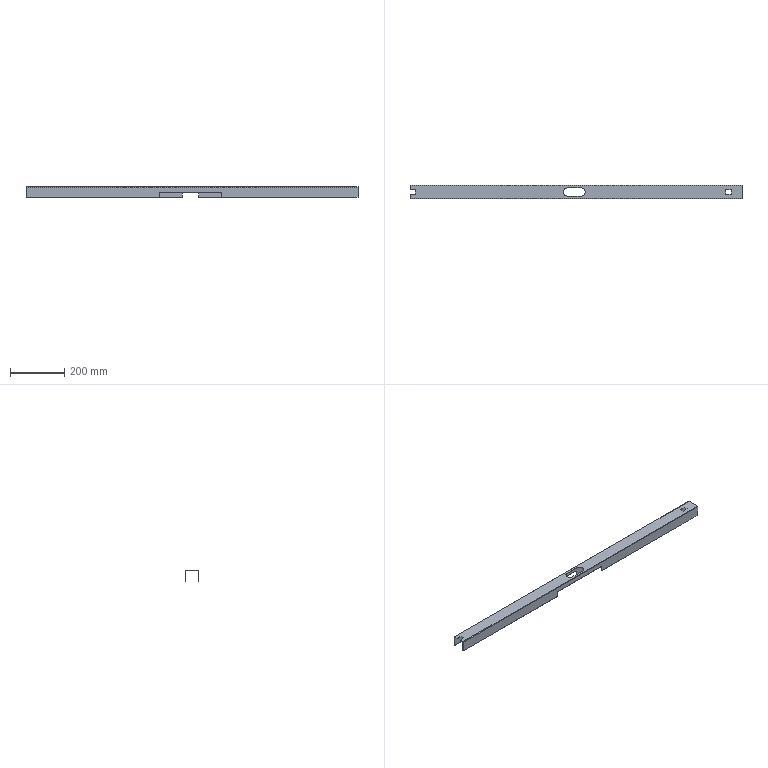Part | 1 solid | 60 faces | box 1222 x 48 x 40 mm | volume 213054 mm3 | plane 44 | cylinder 16 | commonest cylinder face diameters 10 x8 0.4 x2 3.4 x2 6 x2 30 x2